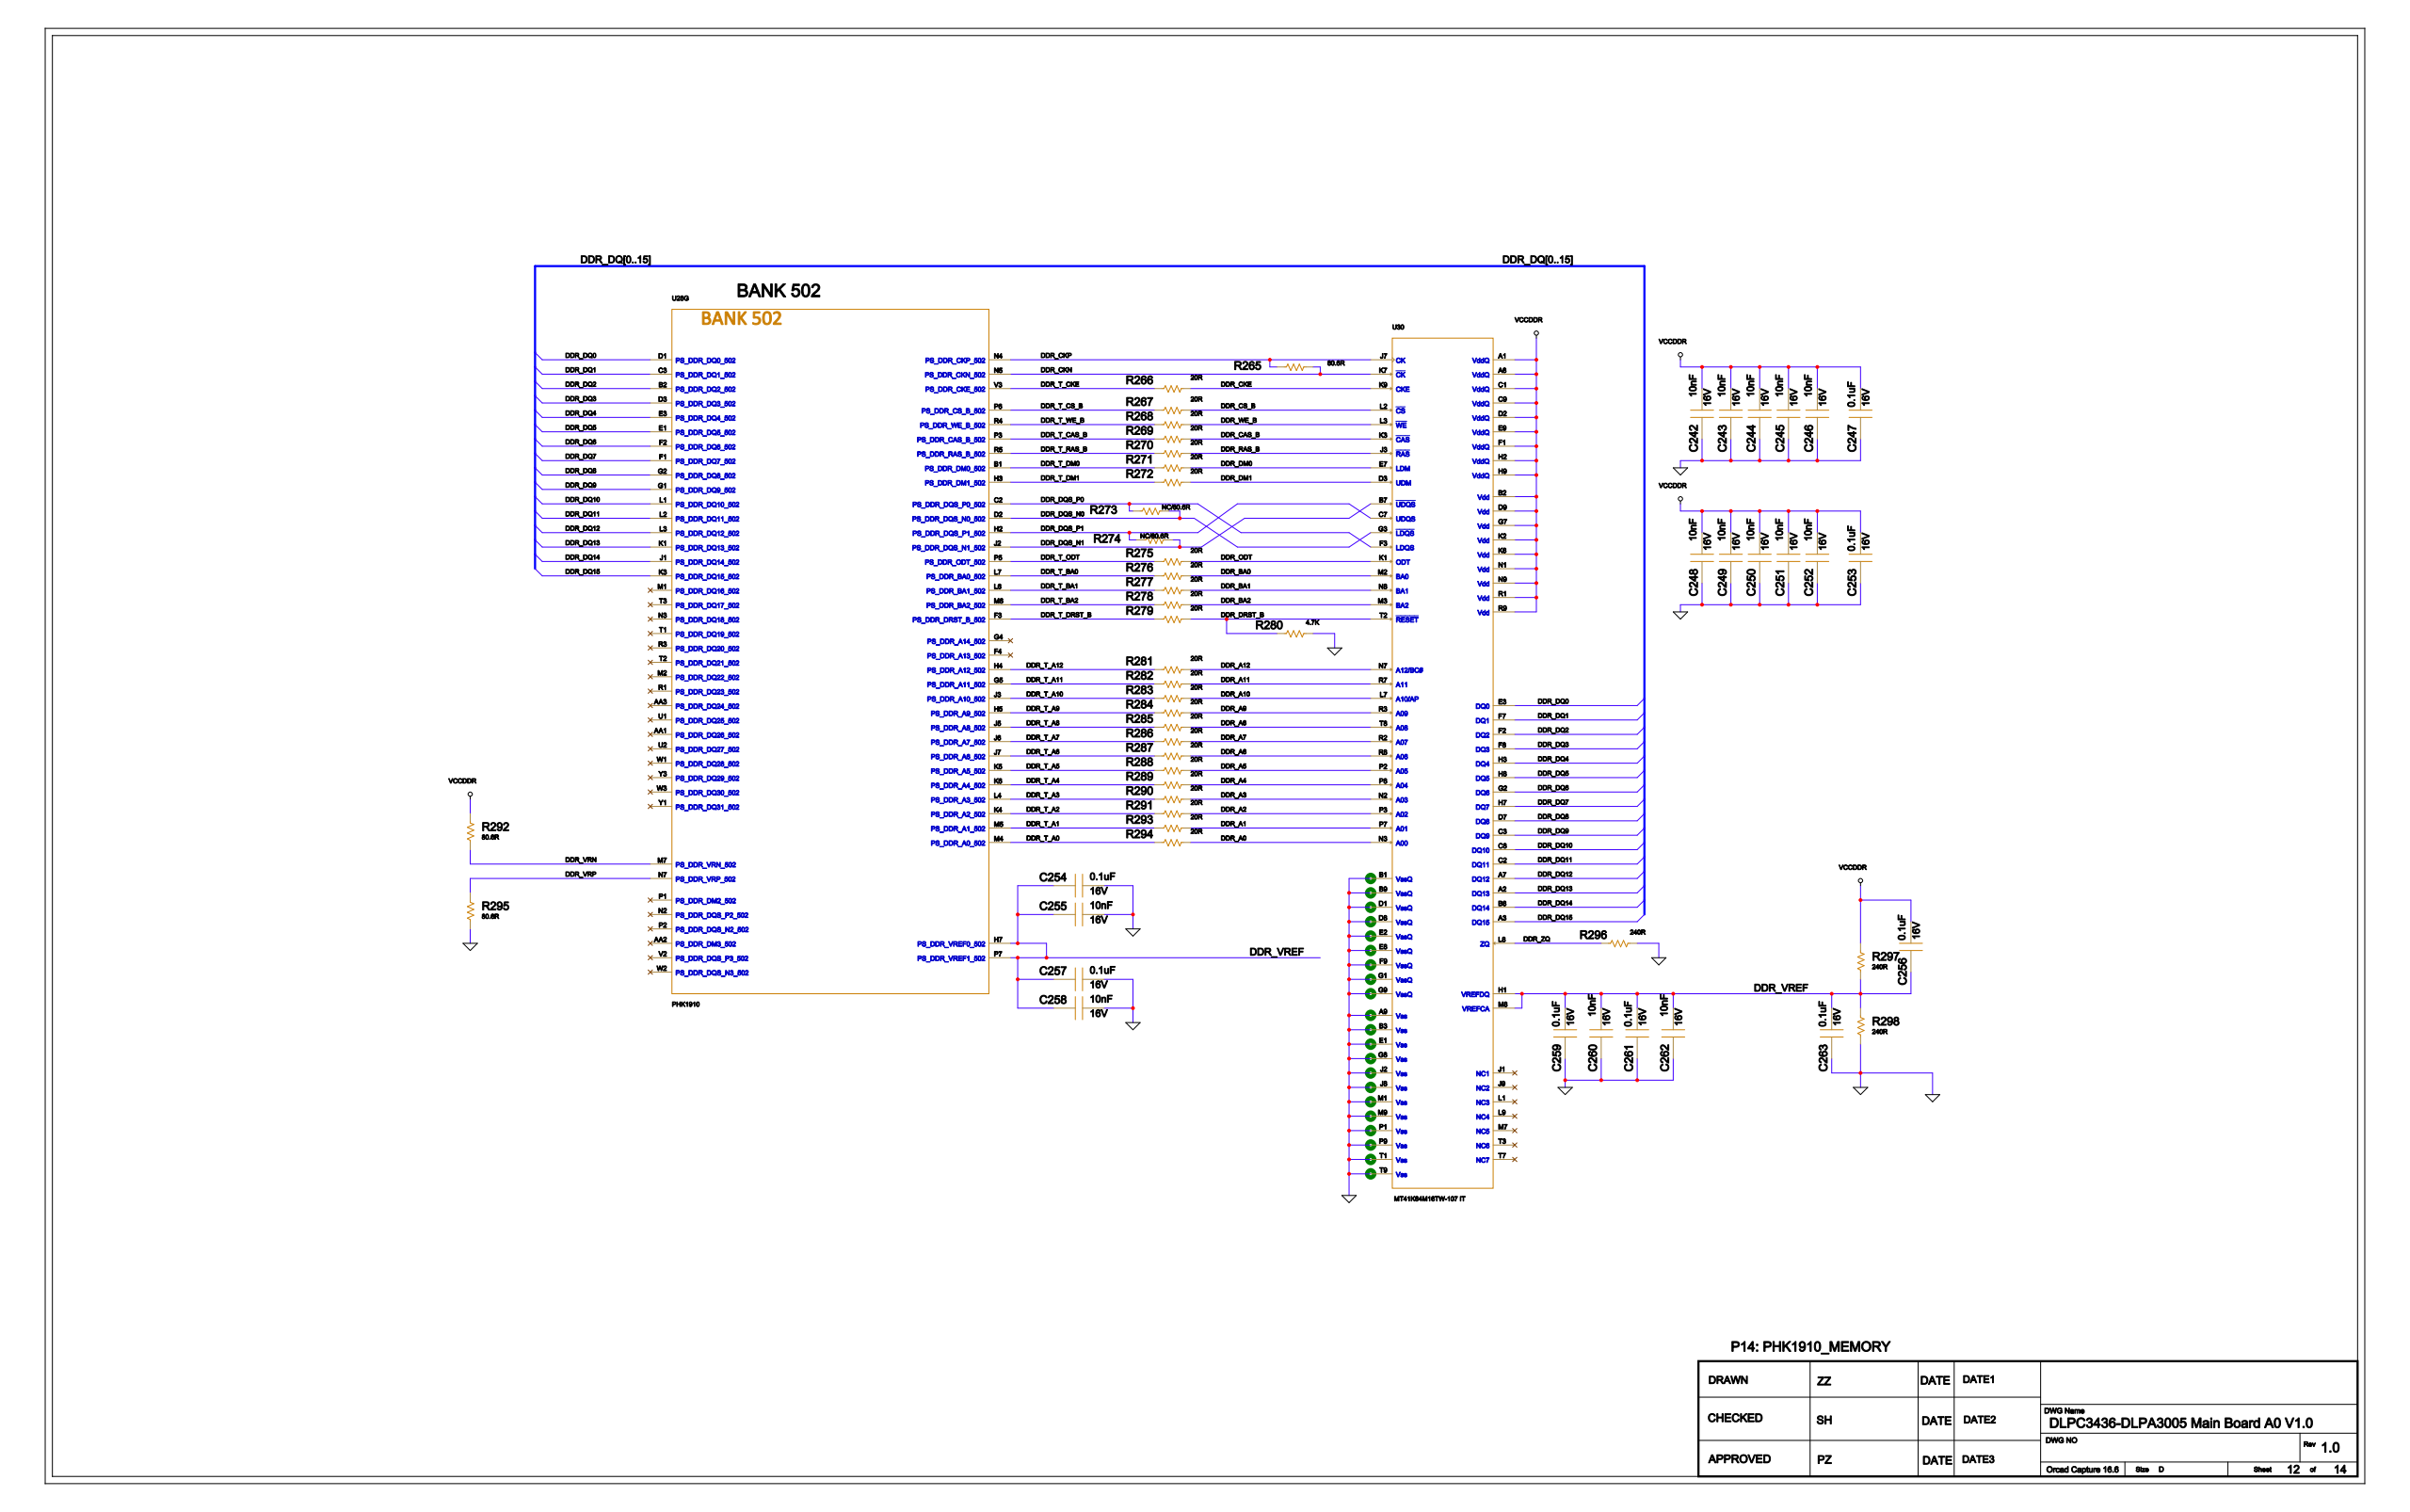Circuit board | Cadence Allegro | 1223 parts | 777 nets | one sheet of the schematic
Parts on this sheet (reference | value | footprint):
C242 | 10nF | C0201
C243 | 10nF | C0201
C244 | 10nF | C0201
C245 | 10nF | C0201
C246 | 10nF | C0201
C247 | 0.1uF | C0201
C248 | 10nF | C0201
C249 | 10nF | C0201
C250 | 10nF | C0201
C251 | 10nF | C0201
C252 | 10nF | C0201
C253 | 0.1uF | C0201
C254 | 0.1uF | C0201
C255 | 10nF | C0201
C256 | 0.1uF | C0201
C257 | 0.1uF | C0201
C258 | 10nF | C0201
C259 | 0.1uF | C0201
C260 | 10nF | C0201
C261 | 0.1uF | C0201
C262 | 10nF | C0201
C263 | 0.1uF | C0201
R265 | 80.6R | R0402
R266 | 20R | R0201
R267 | 20R | R0201
R268 | 20R | R0201
R269 | 20R | R0201
R270 | 20R | R0201
R271 | 20R | R0201
R272 | 20R | R0201
R273 | NC/80.6R | R0402
R274 | NC/80.6R | R0402
R275 | 20R | R0201
R276 | 20R | R0201
R277 | 20R | R0201
R278 | 20R | R0201
R279 | 20R | R0201
R280 | 4.7K | R0201
R281 | 20R | R0201
R282 | 20R | R0201
R283 | 20R | R0201
R284 | 20R | R0201
R285 | 20R | R0201
R286 | 20R | R0201
R287 | 20R | R0201
R288 | 20R | R0201
R289 | 20R | R0201
R290 | 20R | R0201
R291 | 20R | R0201
R292 | 80.6R | R0402
R293 | 20R | R0201
R294 | 20R | R0201
R295 | 80.6R | R0402
R296 | 240R | R0402
R297 | 240R | R0402
R298 | 240R | R0402
U28 | PHK1910 | XILINX_CLG484
U30 | MT41K64M16TW-107 IT | MICRON_96-BALL_FBGA-X16_TW
Nets of these parts (net: part-pin ...):
GND: C242-2 C243-2 C244-2 C245-2 C246-2 C247-2 C248-2 C249-2 C250-2 C251-2 C252-2 C253-2 C254-2 C255-2 C257-2 C258-2 C259-2 C260-2 C261-2 C262-2 C263-2 R280-1 R295-2 R296-1 R298-2 U28-B8 U28-C1 U28-E7 U28-G3 U28-H8 U28-J9 U28-K2 U28-K8 U28-L9 U28-M8 U28-N1 U28-N9 U28-P8 U28-P14 U28-R9 U30-A9 U30-B1 U30-B3 U30-B9 U30-D1 U30-D8 U30-E1 U30-E2 U30-E8 U30-F9 U30-G1 U30-G8 U30-G9 U30-J2 U30-J8 U30-M1 U30-M9 U30-P1 U30-P9 U30-T1 U30-T9
VCCDDR: C242-1 C243-1 C244-1 C245-1 C246-1 C247-1 C248-1 C249-1 C250-1 C251-1 C252-1 C253-1 C256-1 R292-1 R297-1 U28-E2 U28-H1 U28-K7 U28-M3 U28-R2 U30-A1 U30-A8 U30-B2 U30-C1 U30-C9 U30-D2 U30-D9 U30-E9 U30-F1 U30-G7 U30-H2 U30-H9 U30-K2 U30-K8 U30-N1 U30-N9 U30-R1 U30-R9
DDR_VREF: C254-1 C255-1 C256-2 C257-1 C258-1 C259-1 C260-1 C261-1 C262-1 C263-1 R297-2 R298-1 U28-H7 U28-P7 U30-H1 U30-M8
DDR_ZQ: R296-2 U30-L8
DDR_DRST_B: R279-1 R280-2 U30-T2
DDR_CKN: R265-1 U28-N5 U30-K7
DDR_CKP: R265-2 U28-N4 U30-J7
DDR_VRN: R292-2 U28-M7
DDR_VRP: R295-1 U28-N7
DDR_CKE: R266-1 U30-K9
DDR_T_CKE: R266-2 U28-V3
DDR_CS_B: R267-1 U30-L2
DDR_T_CS_B: R267-2 U28-P6
DDR_WE_B: R268-1 U30-L3
DDR_T_WE_B: R268-2 U28-R4
DDR_CAS_B: R269-1 U30-K3
DDR_T_CAS_B: R269-2 U28-P3
DDR_RAS_B: R270-1 U30-J3
DDR_T_RAS_B: R270-2 U28-R5
DDR_DM0: R271-1 U30-E7
DDR_T_DM0: R271-2 U28-B1
DDR_DM1: R272-1 U30-D3
DDR_T_DM1: R272-2 U28-H3
DDR_ODT: R275-1 U30-K1
DDR_T_ODT: R275-2 U28-P5
DDR_BA0: R276-1 U30-M2
DDR_T_BA0: R276-2 U28-L7
DDR_BA1: R277-1 U30-N8
DDR_T_BA1: R277-2 U28-L6
DDR_BA2: R278-1 U30-M3
DDR_T_BA2: R278-2 U28-M6
DDR_T_DRST_B: R279-2 U28-F3
DDR_A12: R281-1 U30-N7
DDR_T_A12: R281-2 U28-H4
DDR_A11: R282-1 U30-R7
DDR_T_A11: R282-2 U28-G5
DDR_A10: R283-1 U30-L7
DDR_T_A10: R283-2 U28-J3
DDR_A9: R284-1 U30-R3
DDR_T_A9: R284-2 U28-H5
DDR_A8: R285-1 U30-T8
DDR_T_A8: R285-2 U28-J5
DDR_A7: R286-1 U30-R2
DDR_T_A7: R286-2 U28-J6
DDR_A6: R287-1 U30-R8
DDR_T_A6: R287-2 U28-J7
DDR_A5: R288-1 U30-P2
DDR_T_A5: R288-2 U28-K5
DDR_A4: R289-1 U30-P8
DDR_T_A4: R289-2 U28-K6
DDR_A3: R290-1 U30-N2
DDR_T_A3: R290-2 U28-L4
DDR_A2: R291-1 U30-P3
DDR_T_A2: R291-2 U28-K4
DDR_A1: R293-1 U30-P7
DDR_T_A1: R293-2 U28-M5
DDR_A0: R294-1 U30-N3
DDR_T_A0: R294-2 U28-M4
DDR_DQS_N0: R273-1 U28-D2 U30-G3
DDR_DQS_P0: R273-2 U28-C2 U30-F3
DDR_DQS_N1: R274-1 U28-J2 U30-B7
DDR_DQS_P1: R274-2 U28-H2 U30-C7
DDR_DQ0: U28-D1 U30-E3
DDR_DQ10: U28-L1 U30-C8
DDR_DQ11: U28-L2 U30-C2
DDR_DQ12: U28-L3 U30-A7
DDR_DQ13: U28-K1 U30-A2
DDR_DQ14: U28-J1 U30-B8
DDR_DQ15: U28-K3 U30-A3
DDR_DQ1: U28-C3 U30-F7
DDR_DQ2: U28-B2 U30-F2
DDR_DQ3: U28-D3 U30-F8
DDR_DQ4: U28-E3 U30-H3
DDR_DQ5: U28-E1 U30-H8
DDR_DQ6: U28-F2 U30-G2
DDR_DQ7: U28-F1 U30-H7
DDR_DQ8: U28-G2 U30-D7
DDR_DQ9: U28-G1 U30-C3